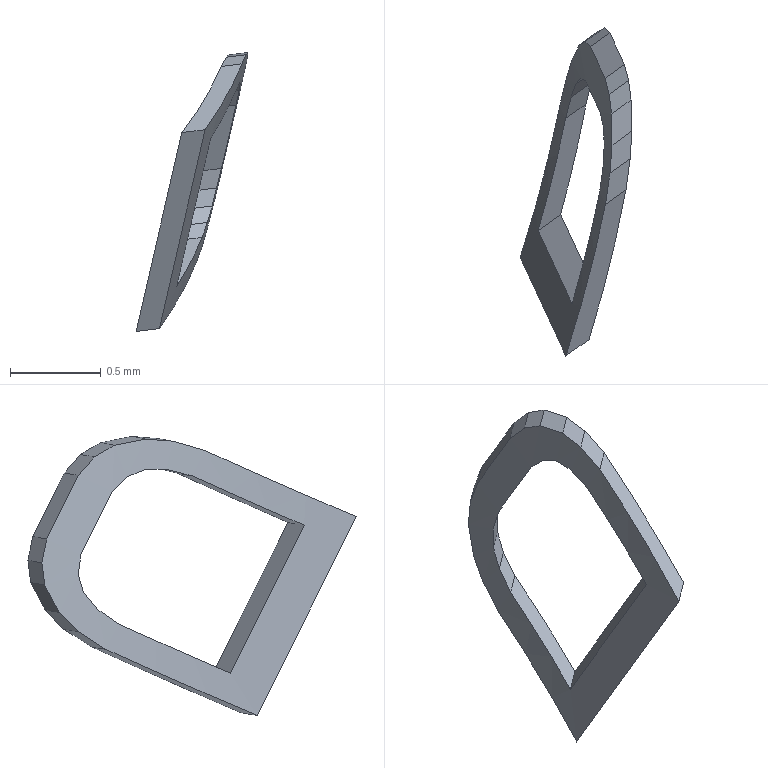Part | SolidWorks | features BaseBody 1 | 1 solid | 28 faces | box 0.6157 x 1.809 x 1.538 mm | volume 0.08303 mm3 | plane 26 | cylinder 2 | commonest cylinder face diameters 16.8 x1 17 x1
STEP:
#1=CARTESIAN_POINT('',(1974.369,-245.081,990.526));
#2=VERTEX_POINT('',#1);
#3=CARTESIAN_POINT('',(1974.587,-244.247,990.891));
#4=VERTEX_POINT('',#3);
#5=CARTESIAN_POINT('',(1966.499,-243.608,993.067));
#6=DIRECTION('',(0.2015,-0.436,0.8771));
#7=DIRECTION('',(-0.7309,-0.6631,-0.1618));
#8=AXIS2_PLACEMENT_3D('',#5,#6,#7);
#9=CIRCLE('',#8,8.4);
#10=EDGE_CURVE('',#2,#4,#9,.T.);
#11=ORIENTED_EDGE('',*,*,#10,.T.);
#12=CARTESIAN_POINT('',(1974.613,-244.073,990.942));
#13=VERTEX_POINT('',#12);
#14=CARTESIAN_POINT('',(1974.587,-244.247,990.891));
#15=CARTESIAN_POINT('',(1974.596,-244.189,990.908));
#16=CARTESIAN_POINT('',(1974.605,-244.131,990.925));
#17=CARTESIAN_POINT('',(1974.613,-244.073,990.942));
#18=B_SPLINE_CURVE_WITH_KNOTS('',3,(#14,#15,#16,#17),.UNSPECIFIED.,.F.,.F.,(4,4),(0.,1.),.UNSPECIFIED.);
#19=EDGE_CURVE('',#4,#13,#18,.T.);
#20=ORIENTED_EDGE('',*,*,#19,.T.);
#21=CARTESIAN_POINT('',(1974.623,-243.921,990.954));
#22=VERTEX_POINT('',#21);
#23=CARTESIAN_POINT('',(1974.613,-244.073,990.942));
#24=CARTESIAN_POINT('',(1974.617,-244.022,990.946));
#25=CARTESIAN_POINT('',(1974.62,-243.972,990.95));
#26=CARTESIAN_POINT('',(1974.623,-243.921,990.954));
#27=B_SPLINE_CURVE_WITH_KNOTS('',3,(#23,#24,#25,#26),.UNSPECIFIED.,.F.,.F.,(4,4),(0.,1.),.UNSPECIFIED.);
#28=EDGE_CURVE('',#13,#22,#27,.T.);
#29=ORIENTED_EDGE('',*,*,#28,.T.);
#30=CARTESIAN_POINT('',(1974.621,-243.748,990.919));
#31=VERTEX_POINT('',#30);
#32=CARTESIAN_POINT('',(1974.623,-243.921,990.954));
#33=CARTESIAN_POINT('',(1974.623,-243.863,990.942));
#34=CARTESIAN_POINT('',(1974.622,-243.806,990.931));
#35=CARTESIAN_POINT('',(1974.621,-243.748,990.919));
#36=B_SPLINE_CURVE_WITH_KNOTS('',3,(#32,#33,#34,#35),.UNSPECIFIED.,.F.,.F.,(4,4),(0.,1.),.UNSPECIFIED.);
#37=EDGE_CURVE('',#22,#31,#36,.T.);
#38=ORIENTED_EDGE('',*,*,#37,.T.);
#39=CARTESIAN_POINT('',(1974.608,-243.639,990.855));
#40=VERTEX_POINT('',#39);
#41=CARTESIAN_POINT('',(1974.621,-243.748,990.919));
#42=CARTESIAN_POINT('',(1974.617,-243.712,990.898));
#43=CARTESIAN_POINT('',(1974.612,-243.675,990.876));
#44=CARTESIAN_POINT('',(1974.608,-243.639,990.855));
#45=B_SPLINE_CURVE_WITH_KNOTS('',3,(#41,#42,#43,#44),.UNSPECIFIED.,.F.,.F.,(4,4),(0.,1.),.UNSPECIFIED.);
#46=EDGE_CURVE('',#31,#40,#45,.T.);
#47=ORIENTED_EDGE('',*,*,#46,.T.);
#48=CARTESIAN_POINT('',(1974.585,-243.55,990.753));
#49=VERTEX_POINT('',#48);
#50=CARTESIAN_POINT('',(1974.608,-243.639,990.855));
#51=CARTESIAN_POINT('',(1974.6,-243.609,990.821));
#52=CARTESIAN_POINT('',(1974.593,-243.58,990.787));
#53=CARTESIAN_POINT('',(1974.585,-243.55,990.753));
#54=B_SPLINE_CURVE_WITH_KNOTS('',3,(#50,#51,#52,#53),.UNSPECIFIED.,.F.,.F.,(4,4),(0.,1.),.UNSPECIFIED.);
#55=EDGE_CURVE('',#40,#49,#54,.T.);
#56=ORIENTED_EDGE('',*,*,#55,.T.);
#57=CARTESIAN_POINT('',(1974.505,-243.376,990.403));
#58=VERTEX_POINT('',#57);
#59=CARTESIAN_POINT('',(1975.622,-245.794,995.266));
#60=DIRECTION('',(-0.2015,0.436,-0.8771));
#61=VECTOR('',#60,1000.);
#62=LINE('',#59,#61);
#63=EDGE_CURVE('',#49,#58,#62,.T.);
#64=ORIENTED_EDGE('',*,*,#63,.T.);
#65=CARTESIAN_POINT('',(1974.474,-243.349,990.272));
#66=VERTEX_POINT('',#65);
#67=CARTESIAN_POINT('',(1974.474,-243.349,990.272));
#68=CARTESIAN_POINT('',(1974.484,-243.358,990.316));
#69=CARTESIAN_POINT('',(1974.495,-243.367,990.359));
#70=CARTESIAN_POINT('',(1974.505,-243.376,990.403));
#71=B_SPLINE_CURVE_WITH_KNOTS('',3,(#67,#68,#69,#70),.UNSPECIFIED.,.F.,.F.,(4,4),(0.,1.),.UNSPECIFIED.);
#72=EDGE_CURVE('',#66,#58,#71,.T.);
#73=ORIENTED_EDGE('',*,*,#72,.F.);
#74=CARTESIAN_POINT('',(1974.444,-243.365,990.149));
#75=VERTEX_POINT('',#74);
#76=CARTESIAN_POINT('',(1974.444,-243.365,990.149));
#77=CARTESIAN_POINT('',(1974.454,-243.36,990.19));
#78=CARTESIAN_POINT('',(1974.464,-243.355,990.231));
#79=CARTESIAN_POINT('',(1974.474,-243.349,990.272));
#80=B_SPLINE_CURVE_WITH_KNOTS('',3,(#76,#77,#78,#79),.UNSPECIFIED.,.F.,.F.,(4,4),(0.,1.),.UNSPECIFIED.);
#81=EDGE_CURVE('',#75,#66,#80,.T.);
#82=ORIENTED_EDGE('',*,*,#81,.F.);
#83=CARTESIAN_POINT('',(1974.404,-243.446,989.998));
#84=VERTEX_POINT('',#83);
#85=CARTESIAN_POINT('',(1974.404,-243.446,989.998));
#86=CARTESIAN_POINT('',(1974.418,-243.419,990.048));
#87=CARTESIAN_POINT('',(1974.431,-243.392,990.099));
#88=CARTESIAN_POINT('',(1974.444,-243.365,990.149));
#89=B_SPLINE_CURVE_WITH_KNOTS('',3,(#85,#86,#87,#88),.UNSPECIFIED.,.F.,.F.,(4,4),(0.,1.),.UNSPECIFIED.);
#90=EDGE_CURVE('',#84,#75,#89,.T.);
#91=ORIENTED_EDGE('',*,*,#90,.F.);
#92=CARTESIAN_POINT('',(1974.371,-243.551,989.892));
#93=VERTEX_POINT('',#92);
#94=CARTESIAN_POINT('',(1974.371,-243.551,989.892));
#95=CARTESIAN_POINT('',(1974.383,-243.516,989.927));
#96=CARTESIAN_POINT('',(1974.393,-243.481,989.962));
#97=CARTESIAN_POINT('',(1974.404,-243.446,989.998));
#98=B_SPLINE_CURVE_WITH_KNOTS('',3,(#94,#95,#96,#97),.UNSPECIFIED.,.F.,.F.,(4,4),(0.,1.),.UNSPECIFIED.);
#99=EDGE_CURVE('',#93,#84,#98,.T.);
#100=ORIENTED_EDGE('',*,*,#99,.F.);
#101=CARTESIAN_POINT('',(1974.335,-243.702,989.795));
#102=VERTEX_POINT('',#101);
#103=CARTESIAN_POINT('',(1974.335,-243.702,989.795));
#104=CARTESIAN_POINT('',(1974.348,-243.652,989.827));
#105=CARTESIAN_POINT('',(1974.36,-243.601,989.859));
#106=CARTESIAN_POINT('',(1974.371,-243.551,989.892));
#107=B_SPLINE_CURVE_WITH_KNOTS('',3,(#103,#104,#105,#106),.UNSPECIFIED.,.F.,.F.,(4,4),(0.,1.),.UNSPECIFIED.);
#108=EDGE_CURVE('',#102,#93,#107,.T.);
#109=ORIENTED_EDGE('',*,*,#108,.F.);
#110=CARTESIAN_POINT('',(1974.117,-244.536,989.43));
#111=VERTEX_POINT('',#110);
#112=CARTESIAN_POINT('',(1966.247,-243.063,991.97));
#113=DIRECTION('',(-0.2015,0.436,-0.8771));
#114=DIRECTION('',(-0.7309,-0.6631,-0.1618));
#115=AXIS2_PLACEMENT_3D('',#112,#113,#114);
#116=CIRCLE('',#115,8.4);
#117=EDGE_CURVE('',#102,#111,#116,.T.);
#118=ORIENTED_EDGE('',*,*,#117,.T.);
#119=CARTESIAN_POINT('',(1975.32,-247.14,994.666));
#120=DIRECTION('',(0.2015,-0.436,0.8771));
#121=VECTOR('',#120,1000.);
#122=LINE('',#119,#121);
#123=EDGE_CURVE('',#111,#2,#122,.T.);
#124=ORIENTED_EDGE('',*,*,#123,.T.);
#125=EDGE_LOOP('',(#11,#20,#29,#38,#47,#56,#64,#73,#82,#91,#100,#109,#118,#124));
#126=FACE_OUTER_BOUND('',#125,.T.);
#127=CARTESIAN_POINT('',(1974.367,-243.772,989.935));
#128=VERTEX_POINT('',#127);
#129=CARTESIAN_POINT('',(1974.398,-243.653,990.017));
#130=VERTEX_POINT('',#129);
#131=CARTESIAN_POINT('',(1974.367,-243.772,989.935));
#132=CARTESIAN_POINT('',(1974.378,-243.732,989.962));
#133=CARTESIAN_POINT('',(1974.388,-243.692,989.99));
#134=CARTESIAN_POINT('',(1974.398,-243.653,990.017));
#135=B_SPLINE_CURVE_WITH_KNOTS('',3,(#131,#132,#133,#134),.UNSPECIFIED.,.F.,.F.,(4,4),(0.,1.),.UNSPECIFIED.);
#136=EDGE_CURVE('',#128,#130,#135,.T.);
#137=ORIENTED_EDGE('',*,*,#136,.T.);
#138=CARTESIAN_POINT('',(1974.425,-243.579,990.108));
#139=VERTEX_POINT('',#138);
#140=CARTESIAN_POINT('',(1974.398,-243.653,990.017));
#141=CARTESIAN_POINT('',(1974.407,-243.628,990.047));
#142=CARTESIAN_POINT('',(1974.416,-243.604,990.078));
#143=CARTESIAN_POINT('',(1974.425,-243.579,990.108));
#144=B_SPLINE_CURVE_WITH_KNOTS('',3,(#140,#141,#142,#143),.UNSPECIFIED.,.F.,.F.,(4,4),(0.,1.),.UNSPECIFIED.);
#145=EDGE_CURVE('',#130,#139,#144,.T.);
#146=ORIENTED_EDGE('',*,*,#145,.T.);
#147=CARTESIAN_POINT('',(1974.452,-243.55,990.208));
#148=VERTEX_POINT('',#147);
#149=CARTESIAN_POINT('',(1974.425,-243.579,990.108));
#150=CARTESIAN_POINT('',(1974.434,-243.569,990.141));
#151=CARTESIAN_POINT('',(1974.443,-243.56,990.174));
#152=CARTESIAN_POINT('',(1974.452,-243.55,990.208));
#153=B_SPLINE_CURVE_WITH_KNOTS('',3,(#149,#150,#151,#152),.UNSPECIFIED.,.F.,.F.,(4,4),(0.,1.),.UNSPECIFIED.);
#154=EDGE_CURVE('',#139,#148,#153,.T.);
#155=ORIENTED_EDGE('',*,*,#154,.T.);
#156=CARTESIAN_POINT('',(1974.478,-243.564,990.315));
#157=VERTEX_POINT('',#156);
#158=CARTESIAN_POINT('',(1974.452,-243.55,990.208));
#159=CARTESIAN_POINT('',(1974.461,-243.555,990.244));
#160=CARTESIAN_POINT('',(1974.47,-243.56,990.279));
#161=CARTESIAN_POINT('',(1974.478,-243.564,990.315));
#162=B_SPLINE_CURVE_WITH_KNOTS('',3,(#158,#159,#160,#161),.UNSPECIFIED.,.F.,.F.,(4,4),(0.,1.),.UNSPECIFIED.);
#163=EDGE_CURVE('',#148,#157,#162,.T.);
#164=ORIENTED_EDGE('',*,*,#163,.T.);
#165=CARTESIAN_POINT('',(1974.559,-243.738,990.665));
#166=VERTEX_POINT('',#165);
#167=CARTESIAN_POINT('',(1975.595,-245.982,995.178));
#168=DIRECTION('',(-0.2015,0.436,-0.8771));
#169=VECTOR('',#168,1000.);
#170=LINE('',#167,#169);
#171=EDGE_CURVE('',#166,#157,#170,.T.);
#172=ORIENTED_EDGE('',*,*,#171,.F.);
#173=CARTESIAN_POINT('',(1974.575,-243.817,990.744));
#174=VERTEX_POINT('',#173);
#175=CARTESIAN_POINT('',(1974.575,-243.817,990.744));
#176=CARTESIAN_POINT('',(1974.57,-243.791,990.718));
#177=CARTESIAN_POINT('',(1974.564,-243.764,990.692));
#178=CARTESIAN_POINT('',(1974.559,-243.738,990.665));
#179=B_SPLINE_CURVE_WITH_KNOTS('',3,(#175,#176,#177,#178),.UNSPECIFIED.,.F.,.F.,(4,4),(0.,1.),.UNSPECIFIED.);
#180=EDGE_CURVE('',#174,#166,#179,.T.);
#181=ORIENTED_EDGE('',*,*,#180,.F.);
#182=CARTESIAN_POINT('',(1974.581,-243.915,990.785));
#183=VERTEX_POINT('',#182);
#184=CARTESIAN_POINT('',(1974.581,-243.915,990.785));
#185=CARTESIAN_POINT('',(1974.579,-243.882,990.771));
#186=CARTESIAN_POINT('',(1974.577,-243.85,990.758));
#187=CARTESIAN_POINT('',(1974.575,-243.817,990.744));
#188=B_SPLINE_CURVE_WITH_KNOTS('',3,(#184,#185,#186,#187),.UNSPECIFIED.,.F.,.F.,(4,4),(0.,1.),.UNSPECIFIED.);
#189=EDGE_CURVE('',#183,#174,#188,.T.);
#190=ORIENTED_EDGE('',*,*,#189,.F.);
#191=CARTESIAN_POINT('',(1974.575,-244.035,990.787));
#192=VERTEX_POINT('',#191);
#193=CARTESIAN_POINT('',(1974.575,-244.035,990.787));
#194=CARTESIAN_POINT('',(1974.577,-243.995,990.786));
#195=CARTESIAN_POINT('',(1974.579,-243.955,990.785));
#196=CARTESIAN_POINT('',(1974.581,-243.915,990.785));
#197=B_SPLINE_CURVE_WITH_KNOTS('',3,(#193,#194,#195,#196),.UNSPECIFIED.,.F.,.F.,(4,4),(0.,1.),.UNSPECIFIED.);
#198=EDGE_CURVE('',#192,#183,#197,.T.);
#199=ORIENTED_EDGE('',*,*,#198,.F.);
#200=CARTESIAN_POINT('',(1974.555,-244.178,990.751));
#201=VERTEX_POINT('',#200);
#202=CARTESIAN_POINT('',(1974.555,-244.178,990.751));
#203=CARTESIAN_POINT('',(1974.562,-244.13,990.763));
#204=CARTESIAN_POINT('',(1974.569,-244.083,990.775));
#205=CARTESIAN_POINT('',(1974.575,-244.035,990.787));
#206=B_SPLINE_CURVE_WITH_KNOTS('',3,(#202,#203,#204,#205),.UNSPECIFIED.,.F.,.F.,(4,4),(0.,1.),.UNSPECIFIED.);
#207=EDGE_CURVE('',#201,#192,#206,.T.);
#208=ORIENTED_EDGE('',*,*,#207,.F.);
#209=CARTESIAN_POINT('',(1974.404,-244.795,990.479));
#210=VERTEX_POINT('',#209);
#211=CARTESIAN_POINT('',(1966.467,-243.538,992.927));
#212=DIRECTION('',(0.2015,-0.436,0.8771));
#213=DIRECTION('',(-0.7309,-0.6631,-0.1618));
#214=AXIS2_PLACEMENT_3D('',#211,#212,#213);
#215=CIRCLE('',#214,8.4);
#216=EDGE_CURVE('',#210,#201,#215,.T.);
#217=ORIENTED_EDGE('',*,*,#216,.F.);
#218=CARTESIAN_POINT('',(1974.216,-244.389,989.663));
#219=VERTEX_POINT('',#218);
#220=CARTESIAN_POINT('',(1975.387,-246.922,994.759));
#221=DIRECTION('',(0.2015,-0.436,0.8771));
#222=VECTOR('',#221,1000.);
#223=LINE('',#220,#222);
#224=EDGE_CURVE('',#219,#210,#223,.T.);
#225=ORIENTED_EDGE('',*,*,#224,.F.);
#226=CARTESIAN_POINT('',(1966.279,-243.133,992.11));
#227=DIRECTION('',(-0.2015,0.436,-0.8771));
#228=DIRECTION('',(-0.7309,-0.6631,-0.1618));
#229=AXIS2_PLACEMENT_3D('',#226,#227,#228);
#230=CIRCLE('',#229,8.4);
#231=EDGE_CURVE('',#128,#219,#230,.T.);
#232=ORIENTED_EDGE('',*,*,#231,.F.);
#233=EDGE_LOOP('',(#137,#146,#155,#164,#172,#181,#190,#199,#208,#217,#225,#232));
#234=FACE_BOUND('',#233,.T.);
#235=CARTESIAN_POINT('',(1967.45,-245.666,997.207));
#236=DIRECTION('',(0.2015,-0.436,0.8771));
#237=DIRECTION('',(-0.7309,-0.6631,-0.1618));
#238=AXIS2_PLACEMENT_3D('',#235,#236,#237);
#239=CYLINDRICAL_SURFACE('',#238,8.4);
#240=ADVANCED_FACE('',(#126,#234),#239,.F.);
#241=CARTESIAN_POINT('',(1974.497,-244.99,990.543));
#242=VERTEX_POINT('',#241);
#243=CARTESIAN_POINT('',(1974.433,-245.036,990.535));
#244=DIRECTION('',(-0.8088,-0.5792,-0.1022));
#245=VECTOR('',#244,1000.);
#246=LINE('',#243,#245);
#247=EDGE_CURVE('',#242,#2,#246,.T.);
#248=ORIENTED_EDGE('',*,*,#247,.T.);
#249=ORIENTED_EDGE('',*,*,#123,.F.);
#250=CARTESIAN_POINT('',(1974.245,-244.445,989.446));
#251=VERTEX_POINT('',#250);
#252=CARTESIAN_POINT('',(1974.181,-244.49,989.438));
#253=DIRECTION('',(-0.8088,-0.5792,-0.1022));
#254=VECTOR('',#253,1000.);
#255=LINE('',#252,#254);
#256=EDGE_CURVE('',#251,#111,#255,.T.);
#257=ORIENTED_EDGE('',*,*,#256,.F.);
#258=CARTESIAN_POINT('',(1974.371,-244.717,989.994));
#259=DIRECTION('',(0.2015,-0.436,0.8771));
#260=VECTOR('',#259,1000.);
#261=LINE('',#258,#260);
#262=EDGE_CURVE('',#251,#242,#261,.T.);
#263=ORIENTED_EDGE('',*,*,#262,.T.);
#264=EDGE_LOOP('',(#248,#249,#257,#263));
#265=FACE_OUTER_BOUND('',#264,.T.);
#266=CARTESIAN_POINT('',(1982.001,-238.89,990.426));
#267=DIRECTION('',(0.5526,-0.6888,-0.4693));
#268=DIRECTION('',(-0.2015,0.436,-0.8771));
#269=AXIS2_PLACEMENT_3D('',#266,#267,#268);
#270=PLANE('',#269);
#271=ADVANCED_FACE('',(#265),#270,.T.);
#272=ORIENTED_EDGE('',*,*,#256,.T.);
#273=ORIENTED_EDGE('',*,*,#117,.F.);
#274=CARTESIAN_POINT('',(1974.449,-243.621,989.809));
#275=VERTEX_POINT('',#274);
#276=CARTESIAN_POINT('',(1974.392,-243.662,989.802));
#277=DIRECTION('',(-0.8088,-0.5792,-0.1022));
#278=VECTOR('',#277,1000.);
#279=LINE('',#276,#278);
#280=EDGE_CURVE('',#275,#102,#279,.T.);
#281=ORIENTED_EDGE('',*,*,#280,.F.);
#282=CARTESIAN_POINT('',(1966.247,-243.063,991.97));
#283=DIRECTION('',(-0.2015,0.436,-0.8771));
#284=DIRECTION('',(-0.7309,-0.6631,-0.1618));
#285=AXIS2_PLACEMENT_3D('',#282,#283,#284);
#286=CIRCLE('',#285,8.5);
#287=EDGE_CURVE('',#275,#251,#286,.T.);
#288=ORIENTED_EDGE('',*,*,#287,.T.);
#289=EDGE_LOOP('',(#272,#273,#281,#288));
#290=FACE_OUTER_BOUND('',#289,.T.);
#291=CARTESIAN_POINT('',(1981.656,-238.46,990.719));
#292=DIRECTION('',(-0.2015,0.436,-0.8771));
#293=DIRECTION('',(-0.5526,0.6888,0.4693));
#294=AXIS2_PLACEMENT_3D('',#291,#292,#293);
#295=PLANE('',#294);
#296=ADVANCED_FACE('',(#290),#295,.T.);
#297=ORIENTED_EDGE('',*,*,#280,.T.);
#298=ORIENTED_EDGE('',*,*,#108,.T.);
#299=CARTESIAN_POINT('',(1974.483,-243.471,989.906));
#300=VERTEX_POINT('',#299);
#301=CARTESIAN_POINT('',(1974.427,-243.511,989.899));
#302=DIRECTION('',(-0.8088,-0.5792,-0.1022));
#303=VECTOR('',#302,1000.);
#304=LINE('',#301,#303);
#305=EDGE_CURVE('',#300,#93,#304,.T.);
#306=ORIENTED_EDGE('',*,*,#305,.F.);
#307=CARTESIAN_POINT('',(1974.449,-243.621,989.809));
#308=CARTESIAN_POINT('',(1974.456,-243.591,989.828));
#309=CARTESIAN_POINT('',(1974.463,-243.561,989.848));
#310=CARTESIAN_POINT('',(1974.47,-243.531,989.867));
#311=CARTESIAN_POINT('',(1974.476,-243.501,989.887));
#312=CARTESIAN_POINT('',(1974.483,-243.471,989.906));
#313=B_SPLINE_CURVE_WITH_KNOTS('',5,(#307,#308,#309,#310,#311,#312),.UNSPECIFIED.,.F.,.F.,(6,6),(0.,1.),.UNSPECIFIED.);
#314=EDGE_CURVE('',#275,#300,#313,.T.);
#315=ORIENTED_EDGE('',*,*,#314,.F.);
#316=EDGE_LOOP('',(#297,#298,#306,#315));
#317=FACE_OUTER_BOUND('',#316,.T.);
#318=CARTESIAN_POINT('',(1981.589,-238.382,990.804));
#319=DIRECTION('',(-0.308,0.5651,-0.7654));
#320=DIRECTION('',(-0.5011,0.5876,0.6354));
#321=AXIS2_PLACEMENT_3D('',#318,#319,#320);
#322=PLANE('',#321);
#323=ADVANCED_FACE('',(#317),#322,.T.);
#324=ORIENTED_EDGE('',*,*,#305,.T.);
#325=ORIENTED_EDGE('',*,*,#99,.T.);
#326=CARTESIAN_POINT('',(1974.513,-243.367,990.011));
#327=VERTEX_POINT('',#326);
#328=CARTESIAN_POINT('',(1974.458,-243.406,990.004));
#329=DIRECTION('',(-0.8088,-0.5792,-0.1022));
#330=VECTOR('',#329,1000.);
#331=LINE('',#328,#330);
#332=EDGE_CURVE('',#327,#84,#331,.T.);
#333=ORIENTED_EDGE('',*,*,#332,.F.);
#334=CARTESIAN_POINT('',(1974.483,-243.471,989.906));
#335=CARTESIAN_POINT('',(1974.489,-243.45,989.927));
#336=CARTESIAN_POINT('',(1974.495,-243.429,989.948));
#337=CARTESIAN_POINT('',(1974.501,-243.409,989.969));
#338=CARTESIAN_POINT('',(1974.507,-243.388,989.99));
#339=CARTESIAN_POINT('',(1974.513,-243.367,990.011));
#340=B_SPLINE_CURVE_WITH_KNOTS('',5,(#334,#335,#336,#337,#338,#339),.UNSPECIFIED.,.F.,.F.,(6,6),(0.,1.),.UNSPECIFIED.);
#341=EDGE_CURVE('',#300,#327,#340,.T.);
#342=ORIENTED_EDGE('',*,*,#341,.F.);
#343=EDGE_LOOP('',(#324,#325,#333,#342));
#344=FACE_OUTER_BOUND('',#343,.T.);
#345=CARTESIAN_POINT('',(1981.542,-238.333,990.899));
#346=DIRECTION('',(-0.4307,0.7016,-0.5677));
#347=DIRECTION('',(-0.4005,0.4151,0.8169));
#348=AXIS2_PLACEMENT_3D('',#345,#346,#347);
#349=PLANE('',#348);
#350=ADVANCED_FACE('',(#344),#349,.T.);
#351=ORIENTED_EDGE('',*,*,#332,.T.);
#352=ORIENTED_EDGE('',*,*,#90,.T.);
#353=CARTESIAN_POINT('',(1974.552,-243.288,990.163));
#354=VERTEX_POINT('',#353);
#355=CARTESIAN_POINT('',(1974.498,-243.327,990.156));
#356=DIRECTION('',(-0.8088,-0.5792,-0.1022));
#357=VECTOR('',#356,1000.);
#358=LINE('',#355,#357);
#359=EDGE_CURVE('',#354,#75,#358,.T.);
#360=ORIENTED_EDGE('',*,*,#359,.F.);
#361=CARTESIAN_POINT('',(1974.513,-243.367,990.011));
#362=CARTESIAN_POINT('',(1974.521,-243.351,990.042));
#363=CARTESIAN_POINT('',(1974.529,-243.335,990.072));
#364=CARTESIAN_POINT('',(1974.537,-243.32,990.102));
#365=CARTESIAN_POINT('',(1974.544,-243.304,990.133));
#366=CARTESIAN_POINT('',(1974.552,-243.288,990.163));
#367=B_SPLINE_CURVE_WITH_KNOTS('',5,(#361,#362,#363,#364,#365,#366),.UNSPECIFIED.,.F.,.F.,(6,6),(0.,1.),.UNSPECIFIED.);
#368=EDGE_CURVE('',#327,#354,#367,.T.);
#369=ORIENTED_EDGE('',*,*,#368,.F.);
#370=EDGE_LOOP('',(#351,#352,#360,#369));
#371=FACE_OUTER_BOUND('',#370,.T.);
#372=CARTESIAN_POINT('',(1981.506,-238.308,991.042));
#373=DIRECTION('',(-0.5358,0.7972,-0.2783));
#374=DIRECTION('',(-0.2426,0.1703,0.955));
#375=AXIS2_PLACEMENT_3D('',#372,#373,#374);
#376=PLANE('',#375);
#377=ADVANCED_FACE('',(#371),#376,.T.);
#378=ORIENTED_EDGE('',*,*,#359,.T.);
#379=ORIENTED_EDGE('',*,*,#81,.T.);
#380=CARTESIAN_POINT('',(1974.581,-243.273,990.285));
#381=VERTEX_POINT('',#380);
#382=CARTESIAN_POINT('',(1974.527,-243.311,990.279));
#383=DIRECTION('',(-0.8088,-0.5792,-0.1022));
#384=VECTOR('',#383,1000.);
#385=LINE('',#382,#384);
#386=EDGE_CURVE('',#381,#66,#385,.T.);
#387=ORIENTED_EDGE('',*,*,#386,.F.);
#388=CARTESIAN_POINT('',(1974.552,-243.288,990.163));
#389=CARTESIAN_POINT('',(1974.558,-243.285,990.188));
#390=CARTESIAN_POINT('',(1974.564,-243.282,990.212));
#391=CARTESIAN_POINT('',(1974.569,-243.279,990.236));
#392=CARTESIAN_POINT('',(1974.575,-243.276,990.261));
#393=CARTESIAN_POINT('',(1974.581,-243.273,990.285));
#394=B_SPLINE_CURVE_WITH_KNOTS('',5,(#388,#389,#390,#391,#392,#393),.UNSPECIFIED.,.F.,.F.,(6,6),(0.,1.),.UNSPECIFIED.);
#395=EDGE_CURVE('',#354,#381,#394,.T.);
#396=ORIENTED_EDGE('',*,*,#395,.F.);
#397=EDGE_LOOP('',(#378,#379,#387,#396));
#398=FACE_OUTER_BOUND('',#397,.T.);
#399=CARTESIAN_POINT('',(1981.499,-238.318,991.159));
#400=DIRECTION('',(-0.5849,0.8103,0.03586));
#401=DIRECTION('',(-0.06203,-0.08877,0.9941));
#402=AXIS2_PLACEMENT_3D('',#399,#400,#401);
#403=PLANE('',#402);
#404=ADVANCED_FACE('',(#398),#403,.T.);
#405=ORIENTED_EDGE('',*,*,#386,.T.);
#406=ORIENTED_EDGE('',*,*,#72,.T.);
#407=CARTESIAN_POINT('',(1974.611,-243.3,990.417));
#408=VERTEX_POINT('',#407);
#409=CARTESIAN_POINT('',(1974.558,-243.338,990.41));
#410=DIRECTION('',(-0.8088,-0.5792,-0.1022));
#411=VECTOR('',#410,1000.);
#412=LINE('',#409,#411);
#413=EDGE_CURVE('',#408,#58,#412,.T.);
#414=ORIENTED_EDGE('',*,*,#413,.F.);
#415=CARTESIAN_POINT('',(1974.581,-243.273,990.285));
#416=CARTESIAN_POINT('',(1974.587,-243.278,990.312));
#417=CARTESIAN_POINT('',(1974.593,-243.283,990.338));
#418=CARTESIAN_POINT('',(1974.599,-243.289,990.364));
#419=CARTESIAN_POINT('',(1974.605,-243.294,990.39));
#420=CARTESIAN_POINT('',(1974.611,-243.3,990.417));
#421=B_SPLINE_CURVE_WITH_KNOTS('',5,(#415,#416,#417,#418,#419,#420),.UNSPECIFIED.,.F.,.F.,(6,6),(0.,1.),.UNSPECIFIED.);
#422=EDGE_CURVE('',#381,#408,#421,.T.);
#423=ORIENTED_EDGE('',*,*,#422,.F.);
#424=EDGE_LOOP('',(#405,#406,#414,#423));
#425=FACE_OUTER_BOUND('',#424,.T.);
#426=CARTESIAN_POINT('',(1981.511,-238.358,991.288));
#427=DIRECTION('',(-0.581,0.7597,0.292));
#428=DIRECTION('',(0.09152,-0.2955,0.9509));
#429=AXIS2_PLACEMENT_3D('',#426,#427,#428);
#430=PLANE('',#429);
#431=ADVANCED_FACE('',(#425),#430,.T.);
#432=ORIENTED_EDGE('',*,*,#413,.T.);
#433=ORIENTED_EDGE('',*,*,#63,.F.);
#434=CARTESIAN_POINT('',(1974.692,-243.474,990.766));
#435=VERTEX_POINT('',#434);
#436=CARTESIAN_POINT('',(1974.638,-243.512,990.76));
#437=DIRECTION('',(-0.8088,-0.5792,-0.1022));
#438=VECTOR('',#437,1000.);
#439=LINE('',#436,#438);
#440=EDGE_CURVE('',#435,#49,#439,.T.);
#441=ORIENTED_EDGE('',*,*,#440,.F.);
#442=CARTESIAN_POINT('',(1974.652,-243.387,990.592));
#443=DIRECTION('',(-0.2015,0.436,-0.8771));
#444=VECTOR('',#443,1000.);
#445=LINE('',#442,#444);
#446=EDGE_CURVE('',#435,#408,#445,.T.);
#447=ORIENTED_EDGE('',*,*,#446,.T.);
#448=EDGE_LOOP('',(#432,#433,#441,#447));
#449=FACE_OUTER_BOUND('',#448,.T.);
#450=CARTESIAN_POINT('',(1981.591,-238.532,991.638));
#451=DIRECTION('',(-0.5526,0.6888,0.4693));
#452=DIRECTION('',(0.2015,-0.436,0.8771));
#453=AXIS2_PLACEMENT_3D('',#450,#451,#452);
#454=PLANE('',#453);
#455=ADVANCED_FACE('',(#449),#454,.T.);
#456=ORIENTED_EDGE('',*,*,#440,.T.);
#457=ORIENTED_EDGE('',*,*,#55,.F.);
#458=CARTESIAN_POINT('',(1974.715,-243.562,990.869));
#459=VERTEX_POINT('',#458);
#460=CARTESIAN_POINT('',(1974.661,-243.601,990.862));
#461=DIRECTION('',(-0.8088,-0.5792,-0.1022));
#462=VECTOR('',#461,1000.);
#463=LINE('',#460,#462);
#464=EDGE_CURVE('',#459,#40,#463,.T.);
#465=ORIENTED_EDGE('',*,*,#464,.F.);
#466=CARTESIAN_POINT('',(1974.715,-243.562,990.869));
#467=CARTESIAN_POINT('',(1974.71,-243.545,990.848));
#468=CARTESIAN_POINT('',(1974.706,-243.527,990.828));
#469=CARTESIAN_POINT('',(1974.701,-243.509,990.807));
#470=CARTESIAN_POINT('',(1974.696,-243.491,990.787));
#471=CARTESIAN_POINT('',(1974.692,-243.474,990.766));
#472=B_SPLINE_CURVE_WITH_KNOTS('',5,(#466,#467,#468,#469,#470,#471),.UNSPECIFIED.,.F.,.F.,(6,6),(0.,1.),.UNSPECIFIED.);
#473=EDGE_CURVE('',#459,#435,#472,.T.);
#474=ORIENTED_EDGE('',*,*,#473,.T.);
#475=EDGE_LOOP('',(#456,#457,#465,#474));
#476=FACE_OUTER_BOUND('',#475,.T.);
#477=CARTESIAN_POINT('',(1981.633,-238.608,991.743));
#478=DIRECTION('',(-0.5035,0.5921,0.6292));
#479=DIRECTION('',(0.3039,-0.5603,0.7705));
#480=AXIS2_PLACEMENT_3D('',#477,#478,#479);
#481=PLANE('',#480);
#482=ADVANCED_FACE('',(#476),#481,.T.);
#483=ORIENTED_EDGE('',*,*,#464,.T.);
#484=ORIENTED_EDGE('',*,*,#46,.F.);
#485=CARTESIAN_POINT('',(1974.729,-243.671,990.933));
#486=VERTEX_POINT('',#485);
#487=CARTESIAN_POINT('',(1974.675,-243.709,990.926));
#488=DIRECTION('',(-0.8088,-0.5792,-0.1022));
#489=VECTOR('',#488,1000.);
#490=LINE('',#487,#489);
#491=EDGE_CURVE('',#486,#31,#490,.T.);
#492=ORIENTED_EDGE('',*,*,#491,.F.);
#493=CARTESIAN_POINT('',(1974.729,-243.671,990.933));
#494=CARTESIAN_POINT('',(1974.726,-243.649,990.92));
#495=CARTESIAN_POINT('',(1974.723,-243.627,990.907));
#496=CARTESIAN_POINT('',(1974.721,-243.606,990.894));
#497=CARTESIAN_POINT('',(1974.718,-243.584,990.881));
#498=CARTESIAN_POINT('',(1974.715,-243.562,990.869));
#499=B_SPLINE_CURVE_WITH_KNOTS('',5,(#493,#494,#495,#496,#497,#498),.UNSPECIFIED.,.F.,.F.,(6,6),(0.,1.),.UNSPECIFIED.);
#500=EDGE_CURVE('',#486,#459,#499,.T.);
#501=ORIENTED_EDGE('',*,*,#500,.T.);
#502=EDGE_LOOP('',(#483,#484,#492,#501));
#503=FACE_OUTER_BOUND('',#502,.T.);
#504=CARTESIAN_POINT('',(1981.683,-238.691,991.811));
#505=DIRECTION('',(-0.4077,0.4269,0.8072));
#506=DIRECTION('',(0.4239,-0.6945,0.5814));
#507=AXIS2_PLACEMENT_3D('',#504,#505,#506);
#508=PLANE('',#507);
#509=ADVANCED_FACE('',(#503),#508,.T.);
#510=ORIENTED_EDGE('',*,*,#491,.T.);
#511=ORIENTED_EDGE('',*,*,#37,.F.);
#512=CARTESIAN_POINT('',(1974.733,-243.843,990.968));
#513=VERTEX_POINT('',#512);
#514=CARTESIAN_POINT('',(1974.678,-243.882,990.961));
#515=DIRECTION('',(-0.8088,-0.5792,-0.1022));
#516=VECTOR('',#515,1000.);
#517=LINE('',#514,#516);
#518=EDGE_CURVE('',#513,#22,#517,.T.);
#519=ORIENTED_EDGE('',*,*,#518,.F.);
#520=CARTESIAN_POINT('',(1974.733,-243.843,990.968));
#521=CARTESIAN_POINT('',(1974.732,-243.808,990.961));
#522=CARTESIAN_POINT('',(1974.732,-243.774,990.954));
#523=CARTESIAN_POINT('',(1974.731,-243.74,990.947));
#524=CARTESIAN_POINT('',(1974.73,-243.705,990.94));
#525=CARTESIAN_POINT('',(1974.729,-243.671,990.933));
#526=B_SPLINE_CURVE_WITH_KNOTS('',5,(#520,#521,#522,#523,#524,#525),.UNSPECIFIED.,.F.,.F.,(6,6),(0.,1.),.UNSPECIFIED.);
#527=EDGE_CURVE('',#513,#486,#526,.T.);
#528=ORIENTED_EDGE('',*,*,#527,.T.);
#529=EDGE_LOOP('',(#510,#511,#519,#528));
#530=FACE_OUTER_BOUND('',#529,.T.);
#531=CARTESIAN_POINT('',(1981.762,-238.809,991.856));
#532=DIRECTION('',(-0.2539,0.1871,0.949));
#533=DIRECTION('',(0.5305,-0.7934,0.2983));
#534=AXIS2_PLACEMENT_3D('',#531,#532,#533);
#535=PLANE('',#534);
#536=ADVANCED_FACE('',(#530),#535,.T.);
#537=ORIENTED_EDGE('',*,*,#518,.T.);
#538=ORIENTED_EDGE('',*,*,#28,.F.);
#539=CARTESIAN_POINT('',(1974.724,-243.993,990.956));
#540=VERTEX_POINT('',#539);
#541=CARTESIAN_POINT('',(1974.668,-244.033,990.949));
#542=DIRECTION('',(-0.8088,-0.5792,-0.1022));
#543=VECTOR('',#542,1000.);
#544=LINE('',#541,#543);
#545=EDGE_CURVE('',#540,#13,#544,.T.);
#546=ORIENTED_EDGE('',*,*,#545,.F.);
#547=CARTESIAN_POINT('',(1974.724,-243.993,990.956));
#548=CARTESIAN_POINT('',(1974.726,-243.963,990.958));
#549=CARTESIAN_POINT('',(1974.728,-243.933,990.961));
#550=CARTESIAN_POINT('',(1974.73,-243.903,990.963));
#551=CARTESIAN_POINT('',(1974.731,-243.873,990.965));
#552=CARTESIAN_POINT('',(1974.733,-243.843,990.968));
#553=B_SPLINE_CURVE_WITH_KNOTS('',5,(#547,#548,#549,#550,#551,#552),.UNSPECIFIED.,.F.,.F.,(6,6),(0.,1.),.UNSPECIFIED.);
#554=EDGE_CURVE('',#540,#513,#553,.T.);
#555=ORIENTED_EDGE('',*,*,#554,.T.);
#556=EDGE_LOOP('',(#537,#538,#546,#555));
#557=FACE_OUTER_BOUND('',#556,.T.);
#558=CARTESIAN_POINT('',(1981.83,-238.904,991.854));
#559=DIRECTION('',(-0.07187,-0.07511,0.9946));
#560=DIRECTION('',(0.5837,-0.8117,-0.01912));
#561=AXIS2_PLACEMENT_3D('',#558,#559,#560);
#562=PLANE('',#561);
#563=ADVANCED_FACE('',(#557),#562,.T.);
#564=ORIENTED_EDGE('',*,*,#545,.T.);
#565=ORIENTED_EDGE('',*,*,#19,.F.);
#566=CARTESIAN_POINT('',(1974.701,-244.166,990.905));
#567=VERTEX_POINT('',#566);
#568=CARTESIAN_POINT('',(1974.644,-244.207,990.898));
#569=DIRECTION('',(-0.8088,-0.5792,-0.1022));
#570=VECTOR('',#569,1000.);
#571=LINE('',#568,#570);
#572=EDGE_CURVE('',#567,#4,#571,.T.);
#573=ORIENTED_EDGE('',*,*,#572,.F.);
#574=CARTESIAN_POINT('',(1974.701,-244.166,990.905));
#575=CARTESIAN_POINT('',(1974.706,-244.132,990.915));
#576=CARTESIAN_POINT('',(1974.711,-244.097,990.925));
#577=CARTESIAN_POINT('',(1974.715,-244.062,990.936));
#578=CARTESIAN_POINT('',(1974.72,-244.028,990.946));
#579=CARTESIAN_POINT('',(1974.724,-243.993,990.956));
#580=B_SPLINE_CURVE_WITH_KNOTS('',5,(#574,#575,#576,#577,#578,#579),.UNSPECIFIED.,.F.,.F.,(6,6),(0.,1.),.UNSPECIFIED.);
#581=EDGE_CURVE('',#567,#540,#580,.T.);
#582=ORIENTED_EDGE('',*,*,#581,.T.);
#583=EDGE_LOOP('',(#564,#565,#573,#582));
#584=FACE_OUTER_BOUND('',#583,.T.);
#585=CARTESIAN_POINT('',(1981.907,-239.005,991.816));
#586=DIRECTION('',(0.08681,-0.2894,0.9533));
#587=DIRECTION('',(0.5817,-0.7621,-0.2843));
#588=AXIS2_PLACEMENT_3D('',#585,#586,#587);
#589=PLANE('',#588);
#590=ADVANCED_FACE('',(#584),#589,.T.);
#591=ORIENTED_EDGE('',*,*,#572,.T.);
#592=ORIENTED_EDGE('',*,*,#10,.F.);
#593=ORIENTED_EDGE('',*,*,#247,.F.);
#594=CARTESIAN_POINT('',(1966.499,-243.608,993.067));
#595=DIRECTION('',(0.2015,-0.436,0.8771));
#596=DIRECTION('',(-0.7309,-0.6631,-0.1618));
#597=AXIS2_PLACEMENT_3D('',#594,#595,#596);
#598=CIRCLE('',#597,8.5);
#599=EDGE_CURVE('',#242,#567,#598,.T.);
#600=ORIENTED_EDGE('',*,*,#599,.T.);
#601=EDGE_LOOP('',(#591,#592,#593,#600));
#602=FACE_OUTER_BOUND('',#601,.T.);
#603=CARTESIAN_POINT('',(1982.253,-239.435,991.522));
#604=DIRECTION('',(0.2015,-0.436,0.8771));
#605=DIRECTION('',(0.5526,-0.6888,-0.4693));
#606=AXIS2_PLACEMENT_3D('',#603,#604,#605);
#607=PLANE('',#606);
#608=ADVANCED_FACE('',(#602),#607,.T.);
#609=CARTESIAN_POINT('',(1974.481,-243.691,989.949));
#610=VERTEX_POINT('',#609);
#611=CARTESIAN_POINT('',(1974.34,-244.3,989.678));
#612=VERTEX_POINT('',#611);
#613=CARTESIAN_POINT('',(1966.279,-243.133,992.11));
#614=DIRECTION('',(-0.2015,0.436,-0.8771));
#615=DIRECTION('',(-0.7309,-0.6631,-0.1618));
#616=AXIS2_PLACEMENT_3D('',#613,#614,#615);
#617=CIRCLE('',#616,8.5);
#618=EDGE_CURVE('',#610,#612,#617,.T.);
#619=ORIENTED_EDGE('',*,*,#618,.F.);
#620=CARTESIAN_POINT('',(1974.424,-243.731,989.942));
#621=DIRECTION('',(-0.8088,-0.5792,-0.1022));
#622=VECTOR('',#621,1000.);
#623=LINE('',#620,#622);
#624=EDGE_CURVE('',#610,#128,#623,.T.);
#625=ORIENTED_EDGE('',*,*,#624,.T.);
#626=ORIENTED_EDGE('',*,*,#231,.T.);
#627=CARTESIAN_POINT('',(1974.278,-244.344,989.671));
#628=DIRECTION('',(-0.8088,-0.5792,-0.1022));
#629=VECTOR('',#628,1000.);
#630=LINE('',#627,#629);
#631=EDGE_CURVE('',#612,#219,#630,.T.);
#632=ORIENTED_EDGE('',*,*,#631,.F.);
#633=EDGE_LOOP('',(#619,#625,#626,#632));
#634=FACE_OUTER_BOUND('',#633,.T.);
#635=CARTESIAN_POINT('',(1981.688,-238.529,990.859));
#636=DIRECTION('',(-0.2015,0.436,-0.8771));
#637=DIRECTION('',(-0.5526,0.6888,0.4693));
#638=AXIS2_PLACEMENT_3D('',#635,#636,#637);
#639=PLANE('',#638);
#640=ADVANCED_FACE('',(#634),#639,.F.);
#641=CARTESIAN_POINT('',(1974.527,-244.706,990.495));
#642=VERTEX_POINT('',#641);
#643=CARTESIAN_POINT('',(1974.434,-244.503,990.087));
#644=DIRECTION('',(0.2015,-0.436,0.8771));
#645=VECTOR('',#644,1000.);
#646=LINE('',#643,#645);
#647=EDGE_CURVE('',#612,#642,#646,.T.);
#648=ORIENTED_EDGE('',*,*,#647,.F.);
#649=ORIENTED_EDGE('',*,*,#631,.T.);
#650=ORIENTED_EDGE('',*,*,#224,.T.);
#651=CARTESIAN_POINT('',(1974.466,-244.75,990.487));
#652=DIRECTION('',(-0.8088,-0.5792,-0.1022));
#653=VECTOR('',#652,1000.);
#654=LINE('',#651,#653);
#655=EDGE_CURVE('',#642,#210,#654,.T.);
#656=ORIENTED_EDGE('',*,*,#655,.F.);
#657=EDGE_LOOP('',(#648,#649,#650,#656));
#658=FACE_OUTER_BOUND('',#657,.T.);
#659=CARTESIAN_POINT('',(1981.947,-238.852,990.639));
#660=DIRECTION('',(0.5526,-0.6888,-0.4693));
#661=DIRECTION('',(-0.2015,0.436,-0.8771));
#662=AXIS2_PLACEMENT_3D('',#659,#660,#661);
#663=PLANE('',#662);
#664=ADVANCED_FACE('',(#658),#663,.F.);
#665=CARTESIAN_POINT('',(1974.669,-244.097,990.765));
#666=VERTEX_POINT('',#665);
#667=CARTESIAN_POINT('',(1966.467,-243.538,992.927));
#668=DIRECTION('',(0.2015,-0.436,0.8771));
#669=DIRECTION('',(-0.7309,-0.6631,-0.1618));
#670=AXIS2_PLACEMENT_3D('',#667,#668,#669);
#671=CIRCLE('',#670,8.5);
#672=EDGE_CURVE('',#642,#666,#671,.T.);
#673=ORIENTED_EDGE('',*,*,#672,.F.);
#674=ORIENTED_EDGE('',*,*,#655,.T.);
#675=ORIENTED_EDGE('',*,*,#216,.T.);
#676=CARTESIAN_POINT('',(1974.612,-244.137,990.758));
#677=DIRECTION('',(-0.8088,-0.5792,-0.1022));
#678=VECTOR('',#677,1000.);
#679=LINE('',#676,#678);
#680=EDGE_CURVE('',#666,#201,#679,.T.);
#681=ORIENTED_EDGE('',*,*,#680,.F.);
#682=EDGE_LOOP('',(#673,#674,#675,#681));
#683=FACE_OUTER_BOUND('',#682,.T.);
#684=CARTESIAN_POINT('',(1982.134,-239.258,991.456));
#685=DIRECTION('',(0.2015,-0.436,0.8771));
#686=DIRECTION('',(0.5526,-0.6888,-0.4693));
#687=AXIS2_PLACEMENT_3D('',#684,#685,#686);
#688=PLANE('',#687);
#689=ADVANCED_FACE('',(#683),#688,.F.);
#690=CARTESIAN_POINT('',(1974.686,-243.955,990.801));
#691=VERTEX_POINT('',#690);
#692=CARTESIAN_POINT('',(1974.669,-244.097,990.765));
#693=CARTESIAN_POINT('',(1974.672,-244.068,990.772));
#694=CARTESIAN_POINT('',(1974.676,-244.04,990.78));
#695=CARTESIAN_POINT('',(1974.68,-244.012,990.787));
#696=CARTESIAN_POINT('',(1974.683,-243.984,990.794));
#697=CARTESIAN_POINT('',(1974.686,-243.955,990.801));
#698=B_SPLINE_CURVE_WITH_KNOTS('',5,(#692,#693,#694,#695,#696,#697),.UNSPECIFIED.,.F.,.F.,(6,6),(0.,1.),.UNSPECIFIED.);
#699=EDGE_CURVE('',#666,#691,#698,.T.);
#700=ORIENTED_EDGE('',*,*,#699,.F.);
#701=ORIENTED_EDGE('',*,*,#680,.T.);
#702=ORIENTED_EDGE('',*,*,#207,.T.);
#703=CARTESIAN_POINT('',(1974.63,-243.995,990.794));
#704=DIRECTION('',(-0.8088,-0.5792,-0.1022));
#705=VECTOR('',#704,1000.);
#706=LINE('',#703,#705);
#707=EDGE_CURVE('',#691,#192,#706,.T.);
#708=ORIENTED_EDGE('',*,*,#707,.F.);
#709=EDGE_LOOP('',(#700,#701,#702,#708));
#710=FACE_OUTER_BOUND('',#709,.T.);
#711=CARTESIAN_POINT('',(1981.875,-238.935,991.676));
#712=DIRECTION('',(0.05851,-0.2521,0.9659));
#713=DIRECTION('',(0.5852,-0.7752,-0.2378));
#714=AXIS2_PLACEMENT_3D('',#711,#712,#713);
#715=PLANE('',#714);
#716=ADVANCED_FACE('',(#710),#715,.F.);
#717=CARTESIAN_POINT('',(1974.691,-243.836,990.799));
#718=VERTEX_POINT('',#717);
#719=CARTESIAN_POINT('',(1974.686,-243.955,990.801));
#720=CARTESIAN_POINT('',(1974.687,-243.932,990.801));
#721=CARTESIAN_POINT('',(1974.688,-243.908,990.8));
#722=CARTESIAN_POINT('',(1974.689,-243.884,990.8));
#723=CARTESIAN_POINT('',(1974.69,-243.86,990.799));
#724=CARTESIAN_POINT('',(1974.691,-243.836,990.799));
#725=B_SPLINE_CURVE_WITH_KNOTS('',5,(#719,#720,#721,#722,#723,#724),.UNSPECIFIED.,.F.,.F.,(6,6),(0.,1.),.UNSPECIFIED.);
#726=EDGE_CURVE('',#691,#718,#725,.T.);
#727=ORIENTED_EDGE('',*,*,#726,.F.);
#728=ORIENTED_EDGE('',*,*,#707,.T.);
#729=ORIENTED_EDGE('',*,*,#198,.T.);
#730=CARTESIAN_POINT('',(1974.636,-243.876,990.792));
#731=DIRECTION('',(-0.8088,-0.5792,-0.1022));
#732=VECTOR('',#731,1000.);
#733=LINE('',#730,#732);
#734=EDGE_CURVE('',#718,#183,#733,.T.);
#735=ORIENTED_EDGE('',*,*,#734,.F.);
#736=EDGE_LOOP('',(#727,#728,#729,#735));
#737=FACE_OUTER_BOUND('',#736,.T.);
#738=CARTESIAN_POINT('',(1981.812,-238.852,991.701));
#739=DIRECTION('',(-0.1444,0.0272,0.9891));
#740=DIRECTION('',(0.5701,-0.8147,0.1057));
#741=AXIS2_PLACEMENT_3D('',#738,#739,#740);
#742=PLANE('',#741);
#743=ADVANCED_FACE('',(#737),#742,.F.);
#744=CARTESIAN_POINT('',(1974.685,-243.738,990.758));
#745=VERTEX_POINT('',#744);
#746=CARTESIAN_POINT('',(1974.691,-243.836,990.799));
#747=CARTESIAN_POINT('',(1974.69,-243.817,990.79));
#748=CARTESIAN_POINT('',(1974.689,-243.797,990.782));
#749=CARTESIAN_POINT('',(1974.687,-243.777,990.774));
#750=CARTESIAN_POINT('',(1974.686,-243.758,990.766));
#751=CARTESIAN_POINT('',(1974.685,-243.738,990.758));
#752=B_SPLINE_CURVE_WITH_KNOTS('',5,(#746,#747,#748,#749,#750,#751),.UNSPECIFIED.,.F.,.F.,(6,6),(0.,1.),.UNSPECIFIED.);
#753=EDGE_CURVE('',#718,#745,#752,.T.);
#754=ORIENTED_EDGE('',*,*,#753,.F.);
#755=ORIENTED_EDGE('',*,*,#734,.T.);
#756=ORIENTED_EDGE('',*,*,#189,.T.);
#757=CARTESIAN_POINT('',(1974.63,-243.777,990.751));
#758=DIRECTION('',(-0.8088,-0.5792,-0.1022));
#759=VECTOR('',#758,1000.);
#760=LINE('',#757,#759);
#761=EDGE_CURVE('',#745,#174,#760,.T.);
#762=ORIENTED_EDGE('',*,*,#761,.F.);
#763=EDGE_LOOP('',(#754,#755,#756,#762));
#764=FACE_OUTER_BOUND('',#763,.T.);
#765=CARTESIAN_POINT('',(1981.759,-238.775,991.691));
#766=DIRECTION('',(-0.3526,0.3384,0.8724));
#767=DIRECTION('',(0.4707,-0.7416,0.4779));
#768=AXIS2_PLACEMENT_3D('',#765,#766,#767);
#769=PLANE('',#768);
#770=ADVANCED_FACE('',(#764),#769,.F.);
#771=CARTESIAN_POINT('',(1974.668,-243.66,990.679));
#772=VERTEX_POINT('',#771);
#773=CARTESIAN_POINT('',(1974.685,-243.738,990.758));
#774=CARTESIAN_POINT('',(1974.681,-243.723,990.742));
#775=CARTESIAN_POINT('',(1974.678,-243.707,990.726));
#776=CARTESIAN_POINT('',(1974.675,-243.691,990.711));
#777=CARTESIAN_POINT('',(1974.671,-243.676,990.695));
#778=CARTESIAN_POINT('',(1974.668,-243.66,990.679));
#779=B_SPLINE_CURVE_WITH_KNOTS('',5,(#773,#774,#775,#776,#777,#778),.UNSPECIFIED.,.F.,.F.,(6,6),(0.,1.),.UNSPECIFIED.);
#780=EDGE_CURVE('',#745,#772,#779,.T.);
#781=ORIENTED_EDGE('',*,*,#780,.F.);
#782=ORIENTED_EDGE('',*,*,#761,.T.);
#783=ORIENTED_EDGE('',*,*,#180,.T.);
#784=CARTESIAN_POINT('',(1974.613,-243.699,990.672));
#785=DIRECTION('',(-0.8088,-0.5792,-0.1022));
#786=VECTOR('',#785,1000.);
#787=LINE('',#784,#786);
#788=EDGE_CURVE('',#772,#166,#787,.T.);
#789=ORIENTED_EDGE('',*,*,#788,.F.);
#790=EDGE_LOOP('',(#781,#782,#783,#789));
#791=FACE_OUTER_BOUND('',#790,.T.);
#792=CARTESIAN_POINT('',(1981.714,-238.704,991.646));
#793=DIRECTION('',(-0.4888,0.5653,0.6644));
#794=DIRECTION('',(0.3271,-0.5873,0.7403));
#795=AXIS2_PLACEMENT_3D('',#792,#793,#794);
#796=PLANE('',#795);
#797=ADVANCED_FACE('',(#791),#796,.F.);
#798=CARTESIAN_POINT('',(1974.587,-243.486,990.329));
#799=VERTEX_POINT('',#798);
#800=CARTESIAN_POINT('',(1974.628,-243.573,990.504));
#801=DIRECTION('',(-0.2015,0.436,-0.8771));
#802=VECTOR('',#801,1000.);
#803=LINE('',#800,#802);
#804=EDGE_CURVE('',#772,#799,#803,.T.);
#805=ORIENTED_EDGE('',*,*,#804,.F.);
#806=ORIENTED_EDGE('',*,*,#788,.T.);
#807=ORIENTED_EDGE('',*,*,#171,.T.);
#808=CARTESIAN_POINT('',(1974.533,-243.525,990.322));
#809=DIRECTION('',(-0.8088,-0.5792,-0.1022));
#810=VECTOR('',#809,1000.);
#811=LINE('',#808,#810);
#812=EDGE_CURVE('',#799,#157,#811,.T.);
#813=ORIENTED_EDGE('',*,*,#812,.F.);
#814=EDGE_LOOP('',(#805,#806,#807,#813));
#815=FACE_OUTER_BOUND('',#814,.T.);
#816=CARTESIAN_POINT('',(1981.678,-238.64,991.565));
#817=DIRECTION('',(-0.5526,0.6888,0.4693));
#818=DIRECTION('',(0.2015,-0.436,0.8771));
#819=AXIS2_PLACEMENT_3D('',#816,#817,#818);
#820=PLANE('',#819);
#821=ADVANCED_FACE('',(#815),#820,.F.);
#822=CARTESIAN_POINT('',(1974.561,-243.471,990.221));
#823=VERTEX_POINT('',#822);
#824=CARTESIAN_POINT('',(1974.561,-243.471,990.221));
#825=CARTESIAN_POINT('',(1974.567,-243.474,990.243));
#826=CARTESIAN_POINT('',(1974.572,-243.477,990.265));
#827=CARTESIAN_POINT('',(1974.577,-243.48,990.286));
#828=CARTESIAN_POINT('',(1974.582,-243.483,990.308));
#829=CARTESIAN_POINT('',(1974.587,-243.486,990.329));
#830=B_SPLINE_CURVE_WITH_KNOTS('',5,(#824,#825,#826,#827,#828,#829),.UNSPECIFIED.,.F.,.F.,(6,6),(0.,1.),.UNSPECIFIED.);
#831=EDGE_CURVE('',#823,#799,#830,.T.);
#832=ORIENTED_EDGE('',*,*,#831,.T.);
#833=ORIENTED_EDGE('',*,*,#812,.T.);
#834=ORIENTED_EDGE('',*,*,#163,.F.);
#835=CARTESIAN_POINT('',(1974.507,-243.511,990.214));
#836=DIRECTION('',(-0.8088,-0.5792,-0.1022));
#837=VECTOR('',#836,1000.);
#838=LINE('',#835,#837);
#839=EDGE_CURVE('',#823,#148,#838,.T.);
#840=ORIENTED_EDGE('',*,*,#839,.F.);
#841=EDGE_LOOP('',(#832,#833,#834,#840));
#842=FACE_OUTER_BOUND('',#841,.T.);
#843=CARTESIAN_POINT('',(1981.597,-238.466,991.215));
#844=DIRECTION('',(-0.5846,0.7727,0.2473));
#845=DIRECTION('',(0.0643,-0.2598,0.9635));
#846=AXIS2_PLACEMENT_3D('',#843,#844,#845);
#847=PLANE('',#846);
#848=ADVANCED_FACE('',(#842),#847,.F.);
#849=CARTESIAN_POINT('',(1974.536,-243.5,990.122));
#850=VERTEX_POINT('',#849);
#851=CARTESIAN_POINT('',(1974.536,-243.5,990.122));
#852=CARTESIAN_POINT('',(1974.541,-243.494,990.142));
#853=CARTESIAN_POINT('',(1974.546,-243.489,990.162));
#854=CARTESIAN_POINT('',(1974.551,-243.483,990.182));
#855=CARTESIAN_POINT('',(1974.556,-243.477,990.201));
#856=CARTESIAN_POINT('',(1974.561,-243.471,990.221));
#857=B_SPLINE_CURVE_WITH_KNOTS('',5,(#851,#852,#853,#854,#855,#856),.UNSPECIFIED.,.F.,.F.,(6,6),(0.,1.),.UNSPECIFIED.);
#858=EDGE_CURVE('',#850,#823,#857,.T.);
#859=ORIENTED_EDGE('',*,*,#858,.T.);
#860=ORIENTED_EDGE('',*,*,#839,.T.);
#861=ORIENTED_EDGE('',*,*,#154,.F.);
#862=CARTESIAN_POINT('',(1974.481,-243.54,990.115));
#863=DIRECTION('',(-0.8088,-0.5792,-0.1022));
#864=VECTOR('',#863,1000.);
#865=LINE('',#862,#864);
#866=EDGE_CURVE('',#850,#139,#865,.T.);
#867=ORIENTED_EDGE('',*,*,#866,.F.);
#868=EDGE_LOOP('',(#859,#860,#861,#867));
#869=FACE_OUTER_BOUND('',#868,.T.);
#870=CARTESIAN_POINT('',(1981.59,-238.438,991.109));
#871=DIRECTION('',(-0.5728,0.8151,-0.08642));
#872=DIRECTION('',(-0.1333,0.01136,0.991));
#873=AXIS2_PLACEMENT_3D('',#870,#871,#872);
#874=PLANE('',#873);
#875=ADVANCED_FACE('',(#869),#874,.F.);
#876=CARTESIAN_POINT('',(1974.509,-243.573,990.031));
#877=VERTEX_POINT('',#876);
#878=CARTESIAN_POINT('',(1974.509,-243.573,990.031));
#879=CARTESIAN_POINT('',(1974.515,-243.558,990.049));
#880=CARTESIAN_POINT('',(1974.52,-243.544,990.068));
#881=CARTESIAN_POINT('',(1974.525,-243.529,990.086));
#882=CARTESIAN_POINT('',(1974.531,-243.515,990.104));
#883=CARTESIAN_POINT('',(1974.536,-243.5,990.122));
#884=B_SPLINE_CURVE_WITH_KNOTS('',5,(#878,#879,#880,#881,#882,#883),.UNSPECIFIED.,.F.,.F.,(6,6),(0.,1.),.UNSPECIFIED.);
#885=EDGE_CURVE('',#877,#850,#884,.T.);
#886=ORIENTED_EDGE('',*,*,#885,.T.);
#887=ORIENTED_EDGE('',*,*,#866,.T.);
#888=ORIENTED_EDGE('',*,*,#145,.F.);
#889=CARTESIAN_POINT('',(1974.454,-243.613,990.024));
#890=DIRECTION('',(-0.8088,-0.5792,-0.1022));
#891=VECTOR('',#890,1000.);
#892=LINE('',#889,#891);
#893=EDGE_CURVE('',#877,#130,#892,.T.);
#894=ORIENTED_EDGE('',*,*,#893,.F.);
#895=EDGE_LOOP('',(#886,#887,#888,#894));
#896=FACE_OUTER_BOUND('',#895,.T.);
#897=CARTESIAN_POINT('',(1981.603,-238.439,991.015));
#898=DIRECTION('',(-0.4775,0.7481,-0.4609));
#899=DIRECTION('',(-0.3434,0.3239,0.8816));
#900=AXIS2_PLACEMENT_3D('',#897,#898,#899);
#901=PLANE('',#900);
#902=ADVANCED_FACE('',(#896),#901,.F.);
#903=CARTESIAN_POINT('',(1974.481,-243.691,989.949));
#904=CARTESIAN_POINT('',(1974.487,-243.667,989.965));
#905=CARTESIAN_POINT('',(1974.493,-243.643,989.982));
#906=CARTESIAN_POINT('',(1974.498,-243.62,989.998));
#907=CARTESIAN_POINT('',(1974.504,-243.596,990.015));
#908=CARTESIAN_POINT('',(1974.509,-243.573,990.031));
#909=B_SPLINE_CURVE_WITH_KNOTS('',5,(#903,#904,#905,#906,#907,#908),.UNSPECIFIED.,.F.,.F.,(6,6),(0.,1.),.UNSPECIFIED.);
#910=EDGE_CURVE('',#610,#877,#909,.T.);
#911=ORIENTED_EDGE('',*,*,#910,.T.);
#912=ORIENTED_EDGE('',*,*,#893,.T.);
#913=ORIENTED_EDGE('',*,*,#136,.F.);
#914=ORIENTED_EDGE('',*,*,#624,.F.);
#915=EDGE_LOOP('',(#911,#912,#913,#914));
#916=FACE_OUTER_BOUND('',#915,.T.);
#917=CARTESIAN_POINT('',(1981.636,-238.469,990.932));
#918=DIRECTION('',(-0.3319,0.5929,-0.7337));
#919=DIRECTION('',(-0.4855,0.5595,0.6717));
#920=AXIS2_PLACEMENT_3D('',#917,#918,#919);
#921=PLANE('',#920);
#922=ADVANCED_FACE('',(#916),#921,.F.);
#923=ORIENTED_EDGE('',*,*,#262,.F.);
#924=ORIENTED_EDGE('',*,*,#287,.F.);
#925=ORIENTED_EDGE('',*,*,#314,.T.);
#926=ORIENTED_EDGE('',*,*,#341,.T.);
#927=ORIENTED_EDGE('',*,*,#368,.T.);
#928=ORIENTED_EDGE('',*,*,#395,.T.);
#929=ORIENTED_EDGE('',*,*,#422,.T.);
#930=ORIENTED_EDGE('',*,*,#446,.F.);
#931=ORIENTED_EDGE('',*,*,#473,.F.);
#932=ORIENTED_EDGE('',*,*,#500,.F.);
#933=ORIENTED_EDGE('',*,*,#527,.F.);
#934=ORIENTED_EDGE('',*,*,#554,.F.);
#935=ORIENTED_EDGE('',*,*,#581,.F.);
#936=ORIENTED_EDGE('',*,*,#599,.F.);
#937=EDGE_LOOP('',(#923,#924,#925,#926,#927,#928,#929,#930,#931,#932,#933,#934,#935,#936));
#938=FACE_OUTER_BOUND('',#937,.T.);
#939=ORIENTED_EDGE('',*,*,#672,.T.);
#940=ORIENTED_EDGE('',*,*,#699,.T.);
#941=ORIENTED_EDGE('',*,*,#726,.T.);
#942=ORIENTED_EDGE('',*,*,#753,.T.);
#943=ORIENTED_EDGE('',*,*,#780,.T.);
#944=ORIENTED_EDGE('',*,*,#804,.T.);
#945=ORIENTED_EDGE('',*,*,#831,.F.);
#946=ORIENTED_EDGE('',*,*,#858,.F.);
#947=ORIENTED_EDGE('',*,*,#885,.F.);
#948=ORIENTED_EDGE('',*,*,#910,.F.);
#949=ORIENTED_EDGE('',*,*,#618,.T.);
#950=ORIENTED_EDGE('',*,*,#647,.T.);
#951=EDGE_LOOP('',(#939,#940,#941,#942,#943,#944,#945,#946,#947,#948,#949,#950));
#952=FACE_BOUND('',#951,.T.);
#953=CARTESIAN_POINT('',(1967.45,-245.666,997.207));
#954=DIRECTION('',(0.2015,-0.436,0.8771));
#955=DIRECTION('',(-0.7309,-0.6631,-0.1618));
#956=AXIS2_PLACEMENT_3D('',#953,#954,#955);
#957=CYLINDRICAL_SURFACE('',#956,8.5);
#958=ADVANCED_FACE('',(#938,#952),#957,.T.);
#959=CLOSED_SHELL('',(#240,#271,#296,#323,#350,#377,#404,#431,#455,#482,#509,#536,#563,#590,#608,#640,#664,#689,#716,#743,#770,#797,#821,#848,#875,#902,#922,#958));
#960=MANIFOLD_SOLID_BREP('',#959);
#961=CARTESIAN_POINT('',(0.,0.,0.));
#962=DIRECTION('',(0.,0.,1.));
#963=DIRECTION('',(1.,0.,0.));
#964=AXIS2_PLACEMENT_3D('',#961,#962,#963);
#965=(LENGTH_UNIT()NAMED_UNIT(*)SI_UNIT(.MILLI.,.METRE.));
#966=UNCERTAINTY_MEASURE_WITH_UNIT(LENGTH_MEASURE(0.00001),#965,'','');
#967=(NAMED_UNIT(*)PLANE_ANGLE_UNIT()SI_UNIT($,.RADIAN.));
#968=(NAMED_UNIT(*)SI_UNIT($,.STERADIAN.)SOLID_ANGLE_UNIT());
#969=(GEOMETRIC_REPRESENTATION_CONTEXT(3)GLOBAL_UNCERTAINTY_ASSIGNED_CONTEXT((#966))GLOBAL_UNIT_ASSIGNED_CONTEXT((#965,#967,#968))REPRESENTATION_CONTEXT('',''));
#970=ADVANCED_BREP_SHAPE_REPRESENTATION('',(#960,#964),#969);